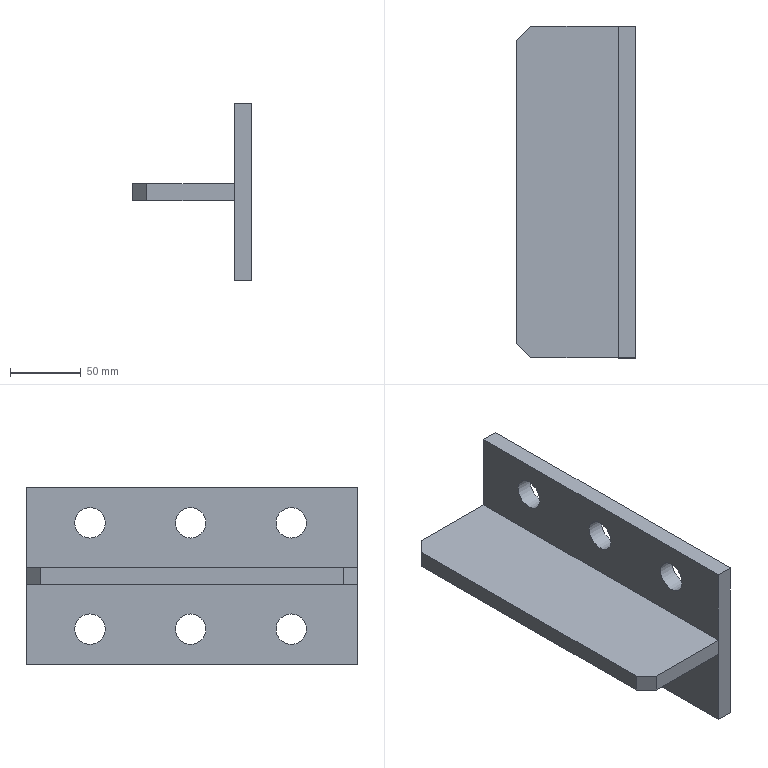Part | STEP file | PN_0028 web-top 12t steel corbel_Default<As Machined> | 2 solids | 20 faces | box 84 x 234 x 125 mm | volume 525836 mm3 | plane 14 | cylinder 6 | commonest cylinder face diameters 21.5 x6
STEP:
#1=CARTESIAN_POINT('',(0.,0.,0.));
#2=DIRECTION('',(0.,0.,1.));
#3=DIRECTION('',(1.,0.,0.));
#4=AXIS2_PLACEMENT_3D('',#1,#2,#3);
#5=CARTESIAN_POINT('',(-26.,117.,0.));
#6=VERTEX_POINT('',#5);
#7=CARTESIAN_POINT('',(-26.,117.,12.));
#8=VERTEX_POINT('',#7);
#9=CARTESIAN_POINT('',(-26.,117.,12.));
#10=DIRECTION('',(0.,0.,1.));
#11=VECTOR('',#10,1.);
#12=LINE('',#9,#11);
#13=CARTESIAN_POINT('',(-26.,117.,12.));
#14=DIRECTION('',(0.7071,-0.7071,0.));
#15=DIRECTION('',(0.,0.,1.));
#16=AXIS2_PLACEMENT_3D('',#13,#14,#15);
#17=PLANE('',#16);
#18=CARTESIAN_POINT('',(0.,0.));
#19=DIRECTION('',(1.,0.));
#20=VECTOR('',#19,1.);
#21=LINE('',#18,#20);
#22=(GEOMETRIC_REPRESENTATION_CONTEXT(2)PARAMETRIC_REPRESENTATION_CONTEXT()REPRESENTATION_CONTEXT('',''));
#23=DEFINITIONAL_REPRESENTATION('',(#21),#22);
#24=PCURVE('',#17,#23);
#25=CARTESIAN_POINT('',(-36.,117.,12.));
#26=DIRECTION('',(0.,-1.,0.));
#27=DIRECTION('',(0.,0.,-1.));
#28=AXIS2_PLACEMENT_3D('',#25,#26,#27);
#29=PLANE('',#28);
#30=CARTESIAN_POINT('',(0.,10.));
#31=DIRECTION('',(-1.,0.));
#32=VECTOR('',#31,1.);
#33=LINE('',#30,#32);
#34=(GEOMETRIC_REPRESENTATION_CONTEXT(2)PARAMETRIC_REPRESENTATION_CONTEXT()REPRESENTATION_CONTEXT('',''));
#35=DEFINITIONAL_REPRESENTATION('',(#33),#34);
#36=PCURVE('',#29,#35);
#37=SURFACE_CURVE('',#12,(#24,#36),.PCURVE_S1.);
#38=EDGE_CURVE('',#6,#8,#37,.T.);
#39=ORIENTED_EDGE('',*,*,#38,.F.);
#40=CARTESIAN_POINT('',(-36.,107.,0.));
#41=VERTEX_POINT('',#40);
#42=CARTESIAN_POINT('',(-26.,117.,0.));
#43=DIRECTION('',(0.7071,0.7071,0.));
#44=VECTOR('',#43,1.);
#45=LINE('',#42,#44);
#46=CARTESIAN_POINT('',(-12.,0.));
#47=DIRECTION('',(0.,-1.));
#48=VECTOR('',#47,1.);
#49=LINE('',#46,#48);
#50=(GEOMETRIC_REPRESENTATION_CONTEXT(2)PARAMETRIC_REPRESENTATION_CONTEXT()REPRESENTATION_CONTEXT('',''));
#51=DEFINITIONAL_REPRESENTATION('',(#49),#50);
#52=PCURVE('',#17,#51);
#53=CARTESIAN_POINT('',(0.,0.,0.));
#54=DIRECTION('',(0.,0.,1.));
#55=DIRECTION('',(1.,0.,0.));
#56=AXIS2_PLACEMENT_3D('',#53,#54,#55);
#57=PLANE('',#56);
#58=CARTESIAN_POINT('',(-26.,117.));
#59=DIRECTION('',(0.7071,0.7071));
#60=VECTOR('',#59,1.);
#61=LINE('',#58,#60);
#62=(GEOMETRIC_REPRESENTATION_CONTEXT(2)PARAMETRIC_REPRESENTATION_CONTEXT()REPRESENTATION_CONTEXT('',''));
#63=DEFINITIONAL_REPRESENTATION('',(#61),#62);
#64=PCURVE('',#57,#63);
#65=SURFACE_CURVE('',#45,(#52,#64),.PCURVE_S1.);
#66=EDGE_CURVE('',#41,#6,#65,.T.);
#67=ORIENTED_EDGE('',*,*,#66,.F.);
#68=CARTESIAN_POINT('',(-36.,107.,12.));
#69=VERTEX_POINT('',#68);
#70=CARTESIAN_POINT('',(-36.,107.,12.));
#71=DIRECTION('',(0.,0.,-1.));
#72=VECTOR('',#71,1.);
#73=LINE('',#70,#72);
#74=CARTESIAN_POINT('',(0.,14.142));
#75=DIRECTION('',(-1.,0.));
#76=VECTOR('',#75,1.);
#77=LINE('',#74,#76);
#78=(GEOMETRIC_REPRESENTATION_CONTEXT(2)PARAMETRIC_REPRESENTATION_CONTEXT()REPRESENTATION_CONTEXT('',''));
#79=DEFINITIONAL_REPRESENTATION('',(#77),#78);
#80=PCURVE('',#17,#79);
#81=CARTESIAN_POINT('',(-36.,117.,12.));
#82=DIRECTION('',(1.,0.,0.));
#83=DIRECTION('',(0.,0.,-1.));
#84=AXIS2_PLACEMENT_3D('',#81,#82,#83);
#85=PLANE('',#84);
#86=CARTESIAN_POINT('',(0.,-10.));
#87=DIRECTION('',(1.,0.));
#88=VECTOR('',#87,1.);
#89=LINE('',#86,#88);
#90=(GEOMETRIC_REPRESENTATION_CONTEXT(2)PARAMETRIC_REPRESENTATION_CONTEXT()REPRESENTATION_CONTEXT('',''));
#91=DEFINITIONAL_REPRESENTATION('',(#89),#90);
#92=PCURVE('',#85,#91);
#93=SURFACE_CURVE('',#73,(#80,#92),.PCURVE_S1.);
#94=EDGE_CURVE('',#69,#41,#93,.T.);
#95=ORIENTED_EDGE('',*,*,#94,.F.);
#96=CARTESIAN_POINT('',(-71.5,71.5,12.));
#97=DIRECTION('',(-0.7071,-0.7071,0.));
#98=VECTOR('',#97,1.);
#99=LINE('',#96,#98);
#100=CARTESIAN_POINT('',(0.,64.347));
#101=DIRECTION('',(0.,1.));
#102=VECTOR('',#101,1.);
#103=LINE('',#100,#102);
#104=(GEOMETRIC_REPRESENTATION_CONTEXT(2)PARAMETRIC_REPRESENTATION_CONTEXT()REPRESENTATION_CONTEXT('',''));
#105=DEFINITIONAL_REPRESENTATION('',(#103),#104);
#106=PCURVE('',#17,#105);
#107=CARTESIAN_POINT('',(0.,0.,12.));
#108=DIRECTION('',(0.,0.,1.));
#109=DIRECTION('',(1.,0.,0.));
#110=AXIS2_PLACEMENT_3D('',#107,#108,#109);
#111=PLANE('',#110);
#112=CARTESIAN_POINT('',(-71.5,71.5));
#113=DIRECTION('',(-0.7071,-0.7071));
#114=VECTOR('',#113,1.);
#115=LINE('',#112,#114);
#116=(GEOMETRIC_REPRESENTATION_CONTEXT(2)PARAMETRIC_REPRESENTATION_CONTEXT()REPRESENTATION_CONTEXT('',''));
#117=DEFINITIONAL_REPRESENTATION('',(#115),#116);
#118=PCURVE('',#111,#117);
#119=SURFACE_CURVE('',#99,(#106,#118),.PCURVE_S1.);
#120=EDGE_CURVE('',#8,#69,#119,.T.);
#121=ORIENTED_EDGE('',*,*,#120,.F.);
#122=EDGE_LOOP('',(#39,#67,#95,#121));
#123=FACE_BOUND('',#122,.T.);
#124=ADVANCED_FACE('',(#123),#17,.F.);
#125=CARTESIAN_POINT('',(-36.,-107.,0.));
#126=VERTEX_POINT('',#125);
#127=CARTESIAN_POINT('',(-36.,-107.,12.));
#128=VERTEX_POINT('',#127);
#129=CARTESIAN_POINT('',(-36.,-107.,12.));
#130=DIRECTION('',(0.,0.,1.));
#131=VECTOR('',#130,1.);
#132=LINE('',#129,#131);
#133=CARTESIAN_POINT('',(-36.,-107.,12.));
#134=DIRECTION('',(0.7071,0.7071,0.));
#135=DIRECTION('',(0.,0.,1.));
#136=AXIS2_PLACEMENT_3D('',#133,#134,#135);
#137=PLANE('',#136);
#138=CARTESIAN_POINT('',(0.,0.));
#139=DIRECTION('',(1.,0.));
#140=VECTOR('',#139,1.);
#141=LINE('',#138,#140);
#142=(GEOMETRIC_REPRESENTATION_CONTEXT(2)PARAMETRIC_REPRESENTATION_CONTEXT()REPRESENTATION_CONTEXT('',''));
#143=DEFINITIONAL_REPRESENTATION('',(#141),#142);
#144=PCURVE('',#137,#143);
#145=CARTESIAN_POINT('',(0.,-224.));
#146=DIRECTION('',(-1.,0.));
#147=VECTOR('',#146,1.);
#148=LINE('',#145,#147);
#149=(GEOMETRIC_REPRESENTATION_CONTEXT(2)PARAMETRIC_REPRESENTATION_CONTEXT()REPRESENTATION_CONTEXT('',''));
#150=DEFINITIONAL_REPRESENTATION('',(#148),#149);
#151=PCURVE('',#85,#150);
#152=SURFACE_CURVE('',#132,(#144,#151),.PCURVE_S1.);
#153=EDGE_CURVE('',#126,#128,#152,.T.);
#154=ORIENTED_EDGE('',*,*,#153,.F.);
#155=CARTESIAN_POINT('',(-26.,-117.,0.));
#156=VERTEX_POINT('',#155);
#157=CARTESIAN_POINT('',(-36.,-107.,0.));
#158=DIRECTION('',(-0.7071,0.7071,0.));
#159=VECTOR('',#158,1.);
#160=LINE('',#157,#159);
#161=CARTESIAN_POINT('',(-12.,0.));
#162=DIRECTION('',(0.,-1.));
#163=VECTOR('',#162,1.);
#164=LINE('',#161,#163);
#165=(GEOMETRIC_REPRESENTATION_CONTEXT(2)PARAMETRIC_REPRESENTATION_CONTEXT()REPRESENTATION_CONTEXT('',''));
#166=DEFINITIONAL_REPRESENTATION('',(#164),#165);
#167=PCURVE('',#137,#166);
#168=CARTESIAN_POINT('',(-36.,-107.));
#169=DIRECTION('',(-0.7071,0.7071));
#170=VECTOR('',#169,1.);
#171=LINE('',#168,#170);
#172=(GEOMETRIC_REPRESENTATION_CONTEXT(2)PARAMETRIC_REPRESENTATION_CONTEXT()REPRESENTATION_CONTEXT('',''));
#173=DEFINITIONAL_REPRESENTATION('',(#171),#172);
#174=PCURVE('',#57,#173);
#175=SURFACE_CURVE('',#160,(#167,#174),.PCURVE_S1.);
#176=EDGE_CURVE('',#156,#126,#175,.T.);
#177=ORIENTED_EDGE('',*,*,#176,.F.);
#178=CARTESIAN_POINT('',(-26.,-117.,12.));
#179=VERTEX_POINT('',#178);
#180=CARTESIAN_POINT('',(-26.,-117.,12.));
#181=DIRECTION('',(0.,0.,-1.));
#182=VECTOR('',#181,1.);
#183=LINE('',#180,#182);
#184=CARTESIAN_POINT('',(0.,14.142));
#185=DIRECTION('',(-1.,0.));
#186=VECTOR('',#185,1.);
#187=LINE('',#184,#186);
#188=(GEOMETRIC_REPRESENTATION_CONTEXT(2)PARAMETRIC_REPRESENTATION_CONTEXT()REPRESENTATION_CONTEXT('',''));
#189=DEFINITIONAL_REPRESENTATION('',(#187),#188);
#190=PCURVE('',#137,#189);
#191=CARTESIAN_POINT('',(-36.,-117.,12.));
#192=DIRECTION('',(0.,1.,0.));
#193=DIRECTION('',(0.,0.,1.));
#194=AXIS2_PLACEMENT_3D('',#191,#192,#193);
#195=PLANE('',#194);
#196=CARTESIAN_POINT('',(0.,10.));
#197=DIRECTION('',(-1.,0.));
#198=VECTOR('',#197,1.);
#199=LINE('',#196,#198);
#200=(GEOMETRIC_REPRESENTATION_CONTEXT(2)PARAMETRIC_REPRESENTATION_CONTEXT()REPRESENTATION_CONTEXT('',''));
#201=DEFINITIONAL_REPRESENTATION('',(#199),#200);
#202=PCURVE('',#195,#201);
#203=SURFACE_CURVE('',#183,(#190,#202),.PCURVE_S1.);
#204=EDGE_CURVE('',#179,#156,#203,.T.);
#205=ORIENTED_EDGE('',*,*,#204,.F.);
#206=CARTESIAN_POINT('',(-71.5,-71.5,12.));
#207=DIRECTION('',(0.7071,-0.7071,0.));
#208=VECTOR('',#207,1.);
#209=LINE('',#206,#208);
#210=CARTESIAN_POINT('',(0.,-50.205));
#211=DIRECTION('',(0.,1.));
#212=VECTOR('',#211,1.);
#213=LINE('',#210,#212);
#214=(GEOMETRIC_REPRESENTATION_CONTEXT(2)PARAMETRIC_REPRESENTATION_CONTEXT()REPRESENTATION_CONTEXT('',''));
#215=DEFINITIONAL_REPRESENTATION('',(#213),#214);
#216=PCURVE('',#137,#215);
#217=CARTESIAN_POINT('',(-71.5,-71.5));
#218=DIRECTION('',(0.7071,-0.7071));
#219=VECTOR('',#218,1.);
#220=LINE('',#217,#219);
#221=(GEOMETRIC_REPRESENTATION_CONTEXT(2)PARAMETRIC_REPRESENTATION_CONTEXT()REPRESENTATION_CONTEXT('',''));
#222=DEFINITIONAL_REPRESENTATION('',(#220),#221);
#223=PCURVE('',#111,#222);
#224=SURFACE_CURVE('',#209,(#216,#223),.PCURVE_S1.);
#225=EDGE_CURVE('',#128,#179,#224,.T.);
#226=ORIENTED_EDGE('',*,*,#225,.F.);
#227=EDGE_LOOP('',(#154,#177,#205,#226));
#228=FACE_BOUND('',#227,.T.);
#229=ADVANCED_FACE('',(#228),#137,.F.);
#230=CARTESIAN_POINT('',(36.,-117.,0.));
#231=VERTEX_POINT('',#230);
#232=CARTESIAN_POINT('',(36.,117.,0.));
#233=VERTEX_POINT('',#232);
#234=CARTESIAN_POINT('',(36.,117.,0.));
#235=DIRECTION('',(0.,1.,0.));
#236=VECTOR('',#235,1.);
#237=LINE('',#234,#236);
#238=CARTESIAN_POINT('',(36.,117.,12.));
#239=DIRECTION('',(-1.,0.,0.));
#240=DIRECTION('',(0.,0.,1.));
#241=AXIS2_PLACEMENT_3D('',#238,#239,#240);
#242=PLANE('',#241);
#243=CARTESIAN_POINT('',(-12.,0.));
#244=DIRECTION('',(0.,1.));
#245=VECTOR('',#244,1.);
#246=LINE('',#243,#245);
#247=(GEOMETRIC_REPRESENTATION_CONTEXT(2)PARAMETRIC_REPRESENTATION_CONTEXT()REPRESENTATION_CONTEXT('',''));
#248=DEFINITIONAL_REPRESENTATION('',(#246),#247);
#249=PCURVE('',#242,#248);
#250=CARTESIAN_POINT('',(36.,117.));
#251=DIRECTION('',(0.,1.));
#252=VECTOR('',#251,1.);
#253=LINE('',#250,#252);
#254=(GEOMETRIC_REPRESENTATION_CONTEXT(2)PARAMETRIC_REPRESENTATION_CONTEXT()REPRESENTATION_CONTEXT('',''));
#255=DEFINITIONAL_REPRESENTATION('',(#253),#254);
#256=PCURVE('',#57,#255);
#257=SURFACE_CURVE('',#237,(#249,#256),.PCURVE_S1.);
#258=EDGE_CURVE('',#231,#233,#257,.T.);
#259=ORIENTED_EDGE('',*,*,#258,.T.);
#260=CARTESIAN_POINT('',(36.,117.,12.));
#261=VERTEX_POINT('',#260);
#262=CARTESIAN_POINT('',(36.,117.,12.));
#263=DIRECTION('',(0.,0.,-1.));
#264=VECTOR('',#263,1.);
#265=LINE('',#262,#264);
#266=CARTESIAN_POINT('',(0.,0.));
#267=DIRECTION('',(-1.,0.));
#268=VECTOR('',#267,1.);
#269=LINE('',#266,#268);
#270=(GEOMETRIC_REPRESENTATION_CONTEXT(2)PARAMETRIC_REPRESENTATION_CONTEXT()REPRESENTATION_CONTEXT('',''));
#271=DEFINITIONAL_REPRESENTATION('',(#269),#270);
#272=PCURVE('',#242,#271);
#273=CARTESIAN_POINT('',(0.,72.));
#274=DIRECTION('',(1.,0.));
#275=VECTOR('',#274,1.);
#276=LINE('',#273,#275);
#277=(GEOMETRIC_REPRESENTATION_CONTEXT(2)PARAMETRIC_REPRESENTATION_CONTEXT()REPRESENTATION_CONTEXT('',''));
#278=DEFINITIONAL_REPRESENTATION('',(#276),#277);
#279=PCURVE('',#29,#278);
#280=SURFACE_CURVE('',#265,(#272,#279),.PCURVE_S1.);
#281=EDGE_CURVE('',#261,#233,#280,.T.);
#282=ORIENTED_EDGE('',*,*,#281,.F.);
#283=CARTESIAN_POINT('',(36.,-117.,12.));
#284=VERTEX_POINT('',#283);
#285=CARTESIAN_POINT('',(36.,117.,12.));
#286=DIRECTION('',(0.,1.,0.));
#287=VECTOR('',#286,1.);
#288=LINE('',#285,#287);
#289=CARTESIAN_POINT('',(0.,0.));
#290=DIRECTION('',(0.,1.));
#291=VECTOR('',#290,1.);
#292=LINE('',#289,#291);
#293=(GEOMETRIC_REPRESENTATION_CONTEXT(2)PARAMETRIC_REPRESENTATION_CONTEXT()REPRESENTATION_CONTEXT('',''));
#294=DEFINITIONAL_REPRESENTATION('',(#292),#293);
#295=PCURVE('',#242,#294);
#296=CARTESIAN_POINT('',(36.,117.));
#297=DIRECTION('',(0.,1.));
#298=VECTOR('',#297,1.);
#299=LINE('',#296,#298);
#300=(GEOMETRIC_REPRESENTATION_CONTEXT(2)PARAMETRIC_REPRESENTATION_CONTEXT()REPRESENTATION_CONTEXT('',''));
#301=DEFINITIONAL_REPRESENTATION('',(#299),#300);
#302=PCURVE('',#111,#301);
#303=SURFACE_CURVE('',#288,(#295,#302),.PCURVE_S1.);
#304=EDGE_CURVE('',#284,#261,#303,.T.);
#305=ORIENTED_EDGE('',*,*,#304,.F.);
#306=CARTESIAN_POINT('',(36.,-117.,12.));
#307=DIRECTION('',(0.,0.,-1.));
#308=VECTOR('',#307,1.);
#309=LINE('',#306,#308);
#310=CARTESIAN_POINT('',(0.,-234.));
#311=DIRECTION('',(-1.,0.));
#312=VECTOR('',#311,1.);
#313=LINE('',#310,#312);
#314=(GEOMETRIC_REPRESENTATION_CONTEXT(2)PARAMETRIC_REPRESENTATION_CONTEXT()REPRESENTATION_CONTEXT('',''));
#315=DEFINITIONAL_REPRESENTATION('',(#313),#314);
#316=PCURVE('',#242,#315);
#317=CARTESIAN_POINT('',(0.,72.));
#318=DIRECTION('',(-1.,0.));
#319=VECTOR('',#318,1.);
#320=LINE('',#317,#319);
#321=(GEOMETRIC_REPRESENTATION_CONTEXT(2)PARAMETRIC_REPRESENTATION_CONTEXT()REPRESENTATION_CONTEXT('',''));
#322=DEFINITIONAL_REPRESENTATION('',(#320),#321);
#323=PCURVE('',#195,#322);
#324=SURFACE_CURVE('',#309,(#316,#323),.PCURVE_S1.);
#325=EDGE_CURVE('',#284,#231,#324,.T.);
#326=ORIENTED_EDGE('',*,*,#325,.T.);
#327=EDGE_LOOP('',(#259,#282,#305,#326));
#328=FACE_BOUND('',#327,.T.);
#329=ADVANCED_FACE('',(#328),#242,.F.);
#330=CARTESIAN_POINT('',(-36.,117.,0.));
#331=DIRECTION('',(-1.,0.,0.));
#332=VECTOR('',#331,1.);
#333=LINE('',#330,#332);
#334=CARTESIAN_POINT('',(12.,0.));
#335=DIRECTION('',(0.,-1.));
#336=VECTOR('',#335,1.);
#337=LINE('',#334,#336);
#338=(GEOMETRIC_REPRESENTATION_CONTEXT(2)PARAMETRIC_REPRESENTATION_CONTEXT()REPRESENTATION_CONTEXT('',''));
#339=DEFINITIONAL_REPRESENTATION('',(#337),#338);
#340=PCURVE('',#29,#339);
#341=CARTESIAN_POINT('',(-36.,117.));
#342=DIRECTION('',(-1.,0.));
#343=VECTOR('',#342,1.);
#344=LINE('',#341,#343);
#345=(GEOMETRIC_REPRESENTATION_CONTEXT(2)PARAMETRIC_REPRESENTATION_CONTEXT()REPRESENTATION_CONTEXT('',''));
#346=DEFINITIONAL_REPRESENTATION('',(#344),#345);
#347=PCURVE('',#57,#346);
#348=SURFACE_CURVE('',#333,(#340,#347),.PCURVE_S1.);
#349=EDGE_CURVE('',#233,#6,#348,.T.);
#350=ORIENTED_EDGE('',*,*,#349,.T.);
#351=ORIENTED_EDGE('',*,*,#38,.T.);
#352=CARTESIAN_POINT('',(-36.,117.,12.));
#353=DIRECTION('',(-1.,0.,0.));
#354=VECTOR('',#353,1.);
#355=LINE('',#352,#354);
#356=CARTESIAN_POINT('',(0.,0.));
#357=DIRECTION('',(0.,-1.));
#358=VECTOR('',#357,1.);
#359=LINE('',#356,#358);
#360=(GEOMETRIC_REPRESENTATION_CONTEXT(2)PARAMETRIC_REPRESENTATION_CONTEXT()REPRESENTATION_CONTEXT('',''));
#361=DEFINITIONAL_REPRESENTATION('',(#359),#360);
#362=PCURVE('',#29,#361);
#363=CARTESIAN_POINT('',(-36.,117.));
#364=DIRECTION('',(-1.,0.));
#365=VECTOR('',#364,1.);
#366=LINE('',#363,#365);
#367=(GEOMETRIC_REPRESENTATION_CONTEXT(2)PARAMETRIC_REPRESENTATION_CONTEXT()REPRESENTATION_CONTEXT('',''));
#368=DEFINITIONAL_REPRESENTATION('',(#366),#367);
#369=PCURVE('',#111,#368);
#370=SURFACE_CURVE('',#355,(#362,#369),.PCURVE_S1.);
#371=EDGE_CURVE('',#261,#8,#370,.T.);
#372=ORIENTED_EDGE('',*,*,#371,.F.);
#373=ORIENTED_EDGE('',*,*,#281,.T.);
#374=EDGE_LOOP('',(#350,#351,#372,#373));
#375=FACE_BOUND('',#374,.T.);
#376=ADVANCED_FACE('',(#375),#29,.F.);
#377=CARTESIAN_POINT('',(-36.,117.,12.));
#378=DIRECTION('',(0.,-1.,0.));
#379=VECTOR('',#378,1.);
#380=LINE('',#377,#379);
#381=CARTESIAN_POINT('',(0.,0.));
#382=DIRECTION('',(0.,-1.));
#383=VECTOR('',#382,1.);
#384=LINE('',#381,#383);
#385=(GEOMETRIC_REPRESENTATION_CONTEXT(2)PARAMETRIC_REPRESENTATION_CONTEXT()REPRESENTATION_CONTEXT('',''));
#386=DEFINITIONAL_REPRESENTATION('',(#384),#385);
#387=PCURVE('',#85,#386);
#388=CARTESIAN_POINT('',(-36.,117.));
#389=DIRECTION('',(0.,-1.));
#390=VECTOR('',#389,1.);
#391=LINE('',#388,#390);
#392=(GEOMETRIC_REPRESENTATION_CONTEXT(2)PARAMETRIC_REPRESENTATION_CONTEXT()REPRESENTATION_CONTEXT('',''));
#393=DEFINITIONAL_REPRESENTATION('',(#391),#392);
#394=PCURVE('',#111,#393);
#395=SURFACE_CURVE('',#380,(#387,#394),.PCURVE_S1.);
#396=EDGE_CURVE('',#69,#128,#395,.T.);
#397=ORIENTED_EDGE('',*,*,#396,.F.);
#398=ORIENTED_EDGE('',*,*,#94,.T.);
#399=CARTESIAN_POINT('',(-36.,117.,0.));
#400=DIRECTION('',(0.,-1.,0.));
#401=VECTOR('',#400,1.);
#402=LINE('',#399,#401);
#403=CARTESIAN_POINT('',(12.,0.));
#404=DIRECTION('',(0.,-1.));
#405=VECTOR('',#404,1.);
#406=LINE('',#403,#405);
#407=(GEOMETRIC_REPRESENTATION_CONTEXT(2)PARAMETRIC_REPRESENTATION_CONTEXT()REPRESENTATION_CONTEXT('',''));
#408=DEFINITIONAL_REPRESENTATION('',(#406),#407);
#409=PCURVE('',#85,#408);
#410=CARTESIAN_POINT('',(-36.,117.));
#411=DIRECTION('',(0.,-1.));
#412=VECTOR('',#411,1.);
#413=LINE('',#410,#412);
#414=(GEOMETRIC_REPRESENTATION_CONTEXT(2)PARAMETRIC_REPRESENTATION_CONTEXT()REPRESENTATION_CONTEXT('',''));
#415=DEFINITIONAL_REPRESENTATION('',(#413),#414);
#416=PCURVE('',#57,#415);
#417=SURFACE_CURVE('',#402,(#409,#416),.PCURVE_S1.);
#418=EDGE_CURVE('',#41,#126,#417,.T.);
#419=ORIENTED_EDGE('',*,*,#418,.T.);
#420=ORIENTED_EDGE('',*,*,#153,.T.);
#421=EDGE_LOOP('',(#397,#398,#419,#420));
#422=FACE_BOUND('',#421,.T.);
#423=ADVANCED_FACE('',(#422),#85,.F.);
#424=CARTESIAN_POINT('',(-36.,-117.,12.));
#425=DIRECTION('',(1.,0.,0.));
#426=VECTOR('',#425,1.);
#427=LINE('',#424,#426);
#428=CARTESIAN_POINT('',(0.,0.));
#429=DIRECTION('',(0.,1.));
#430=VECTOR('',#429,1.);
#431=LINE('',#428,#430);
#432=(GEOMETRIC_REPRESENTATION_CONTEXT(2)PARAMETRIC_REPRESENTATION_CONTEXT()REPRESENTATION_CONTEXT('',''));
#433=DEFINITIONAL_REPRESENTATION('',(#431),#432);
#434=PCURVE('',#195,#433);
#435=CARTESIAN_POINT('',(-36.,-117.));
#436=DIRECTION('',(1.,0.));
#437=VECTOR('',#436,1.);
#438=LINE('',#435,#437);
#439=(GEOMETRIC_REPRESENTATION_CONTEXT(2)PARAMETRIC_REPRESENTATION_CONTEXT()REPRESENTATION_CONTEXT('',''));
#440=DEFINITIONAL_REPRESENTATION('',(#438),#439);
#441=PCURVE('',#111,#440);
#442=SURFACE_CURVE('',#427,(#434,#441),.PCURVE_S1.);
#443=EDGE_CURVE('',#179,#284,#442,.T.);
#444=ORIENTED_EDGE('',*,*,#443,.F.);
#445=ORIENTED_EDGE('',*,*,#204,.T.);
#446=CARTESIAN_POINT('',(-36.,-117.,0.));
#447=DIRECTION('',(1.,0.,0.));
#448=VECTOR('',#447,1.);
#449=LINE('',#446,#448);
#450=CARTESIAN_POINT('',(-12.,0.));
#451=DIRECTION('',(0.,1.));
#452=VECTOR('',#451,1.);
#453=LINE('',#450,#452);
#454=(GEOMETRIC_REPRESENTATION_CONTEXT(2)PARAMETRIC_REPRESENTATION_CONTEXT()REPRESENTATION_CONTEXT('',''));
#455=DEFINITIONAL_REPRESENTATION('',(#453),#454);
#456=PCURVE('',#195,#455);
#457=CARTESIAN_POINT('',(-36.,-117.));
#458=DIRECTION('',(1.,0.));
#459=VECTOR('',#458,1.);
#460=LINE('',#457,#459);
#461=(GEOMETRIC_REPRESENTATION_CONTEXT(2)PARAMETRIC_REPRESENTATION_CONTEXT()REPRESENTATION_CONTEXT('',''));
#462=DEFINITIONAL_REPRESENTATION('',(#460),#461);
#463=PCURVE('',#57,#462);
#464=SURFACE_CURVE('',#449,(#456,#463),.PCURVE_S1.);
#465=EDGE_CURVE('',#156,#231,#464,.T.);
#466=ORIENTED_EDGE('',*,*,#465,.T.);
#467=ORIENTED_EDGE('',*,*,#325,.F.);
#468=EDGE_LOOP('',(#444,#445,#466,#467));
#469=FACE_BOUND('',#468,.T.);
#470=ADVANCED_FACE('',(#469),#195,.F.);
#471=ORIENTED_EDGE('',*,*,#371,.T.);
#472=ORIENTED_EDGE('',*,*,#120,.T.);
#473=ORIENTED_EDGE('',*,*,#396,.T.);
#474=ORIENTED_EDGE('',*,*,#225,.T.);
#475=ORIENTED_EDGE('',*,*,#443,.T.);
#476=ORIENTED_EDGE('',*,*,#304,.T.);
#477=EDGE_LOOP('',(#471,#472,#473,#474,#475,#476));
#478=FACE_BOUND('',#477,.T.);
#479=ADVANCED_FACE('',(#478),#111,.T.);
#480=ORIENTED_EDGE('',*,*,#418,.F.);
#481=ORIENTED_EDGE('',*,*,#66,.T.);
#482=ORIENTED_EDGE('',*,*,#349,.F.);
#483=ORIENTED_EDGE('',*,*,#258,.F.);
#484=ORIENTED_EDGE('',*,*,#465,.F.);
#485=ORIENTED_EDGE('',*,*,#176,.T.);
#486=EDGE_LOOP('',(#480,#481,#482,#483,#484,#485));
#487=FACE_BOUND('',#486,.T.);
#488=ADVANCED_FACE('',(#487),#57,.F.);
#489=CLOSED_SHELL('',(#124,#229,#329,#376,#423,#470,#479,#488));
#490=MANIFOLD_SOLID_BREP('',#489);
#491=CARTESIAN_POINT('',(36.,-117.,-56.496));
#492=VERTEX_POINT('',#491);
#493=CARTESIAN_POINT('',(36.,117.,-56.496));
#494=VERTEX_POINT('',#493);
#495=CARTESIAN_POINT('',(36.,117.,-56.496));
#496=DIRECTION('',(0.,1.,0.));
#497=VECTOR('',#496,1.);
#498=LINE('',#495,#497);
#499=CARTESIAN_POINT('',(48.,117.,-56.496));
#500=DIRECTION('',(0.,0.,1.));
#501=DIRECTION('',(1.,0.,0.));
#502=AXIS2_PLACEMENT_3D('',#499,#500,#501);
#503=PLANE('',#502);
#504=CARTESIAN_POINT('',(-12.,0.));
#505=DIRECTION('',(0.,1.));
#506=VECTOR('',#505,1.);
#507=LINE('',#504,#506);
#508=(GEOMETRIC_REPRESENTATION_CONTEXT(2)PARAMETRIC_REPRESENTATION_CONTEXT()REPRESENTATION_CONTEXT('',''));
#509=DEFINITIONAL_REPRESENTATION('',(#507),#508);
#510=PCURVE('',#503,#509);
#511=CARTESIAN_POINT('',(36.,-17.06,106.06));
#512=DIRECTION('',(1.,0.,0.));
#513=DIRECTION('',(0.,0.,-1.));
#514=AXIS2_PLACEMENT_3D('',#511,#512,#513);
#515=PLANE('',#514);
#516=CARTESIAN_POINT('',(162.556,134.06));
#517=DIRECTION('',(0.,1.));
#518=VECTOR('',#517,1.);
#519=LINE('',#516,#518);
#520=(GEOMETRIC_REPRESENTATION_CONTEXT(2)PARAMETRIC_REPRESENTATION_CONTEXT()REPRESENTATION_CONTEXT('',''));
#521=DEFINITIONAL_REPRESENTATION('',(#519),#520);
#522=PCURVE('',#515,#521);
#523=SURFACE_CURVE('',#498,(#510,#522),.PCURVE_S1.);
#524=EDGE_CURVE('',#492,#494,#523,.T.);
#525=ORIENTED_EDGE('',*,*,#524,.T.);
#526=CARTESIAN_POINT('',(48.,117.,-56.496));
#527=VERTEX_POINT('',#526);
#528=CARTESIAN_POINT('',(48.,117.,-56.496));
#529=DIRECTION('',(-1.,0.,0.));
#530=VECTOR('',#529,1.);
#531=LINE('',#528,#530);
#532=CARTESIAN_POINT('',(0.,0.));
#533=DIRECTION('',(-1.,0.));
#534=VECTOR('',#533,1.);
#535=LINE('',#532,#534);
#536=(GEOMETRIC_REPRESENTATION_CONTEXT(2)PARAMETRIC_REPRESENTATION_CONTEXT()REPRESENTATION_CONTEXT('',''));
#537=DEFINITIONAL_REPRESENTATION('',(#535),#536);
#538=PCURVE('',#503,#537);
#539=CARTESIAN_POINT('',(48.,117.,68.504));
#540=DIRECTION('',(0.,-1.,0.));
#541=DIRECTION('',(0.,0.,-1.));
#542=AXIS2_PLACEMENT_3D('',#539,#540,#541);
#543=PLANE('',#542);
#544=CARTESIAN_POINT('',(125.,0.));
#545=DIRECTION('',(0.,-1.));
#546=VECTOR('',#545,1.);
#547=LINE('',#544,#546);
#548=(GEOMETRIC_REPRESENTATION_CONTEXT(2)PARAMETRIC_REPRESENTATION_CONTEXT()REPRESENTATION_CONTEXT('',''));
#549=DEFINITIONAL_REPRESENTATION('',(#547),#548);
#550=PCURVE('',#543,#549);
#551=SURFACE_CURVE('',#531,(#538,#550),.PCURVE_S1.);
#552=EDGE_CURVE('',#527,#494,#551,.T.);
#553=ORIENTED_EDGE('',*,*,#552,.F.);
#554=CARTESIAN_POINT('',(48.,-117.,-56.496));
#555=VERTEX_POINT('',#554);
#556=CARTESIAN_POINT('',(48.,117.,-56.496));
#557=DIRECTION('',(0.,1.,0.));
#558=VECTOR('',#557,1.);
#559=LINE('',#556,#558);
#560=CARTESIAN_POINT('',(0.,0.));
#561=DIRECTION('',(0.,1.));
#562=VECTOR('',#561,1.);
#563=LINE('',#560,#562);
#564=(GEOMETRIC_REPRESENTATION_CONTEXT(2)PARAMETRIC_REPRESENTATION_CONTEXT()REPRESENTATION_CONTEXT('',''));
#565=DEFINITIONAL_REPRESENTATION('',(#563),#564);
#566=PCURVE('',#503,#565);
#567=CARTESIAN_POINT('',(48.,-17.06,106.06));
#568=DIRECTION('',(1.,0.,0.));
#569=DIRECTION('',(0.,0.,-1.));
#570=AXIS2_PLACEMENT_3D('',#567,#568,#569);
#571=PLANE('',#570);
#572=CARTESIAN_POINT('',(162.556,134.06));
#573=DIRECTION('',(0.,1.));
#574=VECTOR('',#573,1.);
#575=LINE('',#572,#574);
#576=(GEOMETRIC_REPRESENTATION_CONTEXT(2)PARAMETRIC_REPRESENTATION_CONTEXT()REPRESENTATION_CONTEXT('',''));
#577=DEFINITIONAL_REPRESENTATION('',(#575),#576);
#578=PCURVE('',#571,#577);
#579=SURFACE_CURVE('',#559,(#566,#578),.PCURVE_S1.);
#580=EDGE_CURVE('',#555,#527,#579,.T.);
#581=ORIENTED_EDGE('',*,*,#580,.F.);
#582=CARTESIAN_POINT('',(48.,-117.,-56.496));
#583=DIRECTION('',(-1.,0.,0.));
#584=VECTOR('',#583,1.);
#585=LINE('',#582,#584);
#586=CARTESIAN_POINT('',(0.,-234.));
#587=DIRECTION('',(-1.,0.));
#588=VECTOR('',#587,1.);
#589=LINE('',#586,#588);
#590=(GEOMETRIC_REPRESENTATION_CONTEXT(2)PARAMETRIC_REPRESENTATION_CONTEXT()REPRESENTATION_CONTEXT('',''));
#591=DEFINITIONAL_REPRESENTATION('',(#589),#590);
#592=PCURVE('',#503,#591);
#593=CARTESIAN_POINT('',(48.,-117.,68.504));
#594=DIRECTION('',(0.,1.,0.));
#595=DIRECTION('',(0.,0.,1.));
#596=AXIS2_PLACEMENT_3D('',#593,#594,#595);
#597=PLANE('',#596);
#598=CARTESIAN_POINT('',(-125.,0.));
#599=DIRECTION('',(0.,-1.));
#600=VECTOR('',#599,1.);
#601=LINE('',#598,#600);
#602=(GEOMETRIC_REPRESENTATION_CONTEXT(2)PARAMETRIC_REPRESENTATION_CONTEXT()REPRESENTATION_CONTEXT('',''));
#603=DEFINITIONAL_REPRESENTATION('',(#601),#602);
#604=PCURVE('',#597,#603);
#605=SURFACE_CURVE('',#585,(#592,#604),.PCURVE_S1.);
#606=EDGE_CURVE('',#555,#492,#605,.T.);
#607=ORIENTED_EDGE('',*,*,#606,.T.);
#608=EDGE_LOOP('',(#525,#553,#581,#607));
#609=FACE_BOUND('',#608,.T.);
#610=ADVANCED_FACE('',(#609),#503,.F.);
#611=CARTESIAN_POINT('',(36.,117.,68.504));
#612=VERTEX_POINT('',#611);
#613=CARTESIAN_POINT('',(36.,117.,68.504));
#614=DIRECTION('',(0.,0.,1.));
#615=VECTOR('',#614,1.);
#616=LINE('',#613,#615);
#617=CARTESIAN_POINT('',(0.,-12.));
#618=DIRECTION('',(-1.,0.));
#619=VECTOR('',#618,1.);
#620=LINE('',#617,#619);
#621=(GEOMETRIC_REPRESENTATION_CONTEXT(2)PARAMETRIC_REPRESENTATION_CONTEXT()REPRESENTATION_CONTEXT('',''));
#622=DEFINITIONAL_REPRESENTATION('',(#620),#621);
#623=PCURVE('',#543,#622);
#624=CARTESIAN_POINT('',(37.556,134.06));
#625=DIRECTION('',(-1.,0.));
#626=VECTOR('',#625,1.);
#627=LINE('',#624,#626);
#628=(GEOMETRIC_REPRESENTATION_CONTEXT(2)PARAMETRIC_REPRESENTATION_CONTEXT()REPRESENTATION_CONTEXT('',''));
#629=DEFINITIONAL_REPRESENTATION('',(#627),#628);
#630=PCURVE('',#515,#629);
#631=SURFACE_CURVE('',#616,(#623,#630),.PCURVE_S1.);
#632=EDGE_CURVE('',#494,#612,#631,.T.);
#633=ORIENTED_EDGE('',*,*,#632,.T.);
#634=CARTESIAN_POINT('',(48.,117.,68.504));
#635=VERTEX_POINT('',#634);
#636=CARTESIAN_POINT('',(48.,117.,68.504));
#637=DIRECTION('',(-1.,0.,0.));
#638=VECTOR('',#637,1.);
#639=LINE('',#636,#638);
#640=CARTESIAN_POINT('',(0.,0.));
#641=DIRECTION('',(0.,-1.));
#642=VECTOR('',#641,1.);
#643=LINE('',#640,#642);
#644=(GEOMETRIC_REPRESENTATION_CONTEXT(2)PARAMETRIC_REPRESENTATION_CONTEXT()REPRESENTATION_CONTEXT('',''));
#645=DEFINITIONAL_REPRESENTATION('',(#643),#644);
#646=PCURVE('',#543,#645);
#647=CARTESIAN_POINT('',(48.,117.,68.504));
#648=DIRECTION('',(0.,0.,-1.));
#649=DIRECTION('',(0.,1.,0.));
#650=AXIS2_PLACEMENT_3D('',#647,#648,#649);
#651=PLANE('',#650);
#652=CARTESIAN_POINT('',(0.,0.));
#653=DIRECTION('',(0.,-1.));
#654=VECTOR('',#653,1.);
#655=LINE('',#652,#654);
#656=(GEOMETRIC_REPRESENTATION_CONTEXT(2)PARAMETRIC_REPRESENTATION_CONTEXT()REPRESENTATION_CONTEXT('',''));
#657=DEFINITIONAL_REPRESENTATION('',(#655),#656);
#658=PCURVE('',#651,#657);
#659=SURFACE_CURVE('',#639,(#646,#658),.PCURVE_S1.);
#660=EDGE_CURVE('',#635,#612,#659,.T.);
#661=ORIENTED_EDGE('',*,*,#660,.F.);
#662=CARTESIAN_POINT('',(48.,117.,68.504));
#663=DIRECTION('',(0.,0.,1.));
#664=VECTOR('',#663,1.);
#665=LINE('',#662,#664);
#666=CARTESIAN_POINT('',(0.,0.));
#667=DIRECTION('',(-1.,0.));
#668=VECTOR('',#667,1.);
#669=LINE('',#666,#668);
#670=(GEOMETRIC_REPRESENTATION_CONTEXT(2)PARAMETRIC_REPRESENTATION_CONTEXT()REPRESENTATION_CONTEXT('',''));
#671=DEFINITIONAL_REPRESENTATION('',(#669),#670);
#672=PCURVE('',#543,#671);
#673=CARTESIAN_POINT('',(37.556,134.06));
#674=DIRECTION('',(-1.,0.));
#675=VECTOR('',#674,1.);
#676=LINE('',#673,#675);
#677=(GEOMETRIC_REPRESENTATION_CONTEXT(2)PARAMETRIC_REPRESENTATION_CONTEXT()REPRESENTATION_CONTEXT('',''));
#678=DEFINITIONAL_REPRESENTATION('',(#676),#677);
#679=PCURVE('',#571,#678);
#680=SURFACE_CURVE('',#665,(#672,#679),.PCURVE_S1.);
#681=EDGE_CURVE('',#527,#635,#680,.T.);
#682=ORIENTED_EDGE('',*,*,#681,.F.);
#683=ORIENTED_EDGE('',*,*,#552,.T.);
#684=EDGE_LOOP('',(#633,#661,#682,#683));
#685=FACE_BOUND('',#684,.T.);
#686=ADVANCED_FACE('',(#685),#543,.F.);
#687=CARTESIAN_POINT('',(36.,-117.,68.504));
#688=VERTEX_POINT('',#687);
#689=CARTESIAN_POINT('',(36.,117.,68.504));
#690=DIRECTION('',(0.,-1.,0.));
#691=VECTOR('',#690,1.);
#692=LINE('',#689,#691);
#693=CARTESIAN_POINT('',(0.,-12.));
#694=DIRECTION('',(-1.,0.));
#695=VECTOR('',#694,1.);
#696=LINE('',#693,#695);
#697=(GEOMETRIC_REPRESENTATION_CONTEXT(2)PARAMETRIC_REPRESENTATION_CONTEXT()REPRESENTATION_CONTEXT('',''));
#698=DEFINITIONAL_REPRESENTATION('',(#696),#697);
#699=PCURVE('',#651,#698);
#700=CARTESIAN_POINT('',(37.556,134.06));
#701=DIRECTION('',(0.,-1.));
#702=VECTOR('',#701,1.);
#703=LINE('',#700,#702);
#704=(GEOMETRIC_REPRESENTATION_CONTEXT(2)PARAMETRIC_REPRESENTATION_CONTEXT()REPRESENTATION_CONTEXT('',''));
#705=DEFINITIONAL_REPRESENTATION('',(#703),#704);
#706=PCURVE('',#515,#705);
#707=SURFACE_CURVE('',#692,(#699,#706),.PCURVE_S1.);
#708=EDGE_CURVE('',#612,#688,#707,.T.);
#709=ORIENTED_EDGE('',*,*,#708,.T.);
#710=CARTESIAN_POINT('',(48.,-117.,68.504));
#711=VERTEX_POINT('',#710);
#712=CARTESIAN_POINT('',(48.,-117.,68.504));
#713=DIRECTION('',(-1.,0.,0.));
#714=VECTOR('',#713,1.);
#715=LINE('',#712,#714);
#716=CARTESIAN_POINT('',(-234.,0.));
#717=DIRECTION('',(0.,-1.));
#718=VECTOR('',#717,1.);
#719=LINE('',#716,#718);
#720=(GEOMETRIC_REPRESENTATION_CONTEXT(2)PARAMETRIC_REPRESENTATION_CONTEXT()REPRESENTATION_CONTEXT('',''));
#721=DEFINITIONAL_REPRESENTATION('',(#719),#720);
#722=PCURVE('',#651,#721);
#723=CARTESIAN_POINT('',(0.,0.));
#724=DIRECTION('',(0.,-1.));
#725=VECTOR('',#724,1.);
#726=LINE('',#723,#725);
#727=(GEOMETRIC_REPRESENTATION_CONTEXT(2)PARAMETRIC_REPRESENTATION_CONTEXT()REPRESENTATION_CONTEXT('',''));
#728=DEFINITIONAL_REPRESENTATION('',(#726),#727);
#729=PCURVE('',#597,#728);
#730=SURFACE_CURVE('',#715,(#722,#729),.PCURVE_S1.);
#731=EDGE_CURVE('',#711,#688,#730,.T.);
#732=ORIENTED_EDGE('',*,*,#731,.F.);
#733=CARTESIAN_POINT('',(48.,117.,68.504));
#734=DIRECTION('',(0.,-1.,0.));
#735=VECTOR('',#734,1.);
#736=LINE('',#733,#735);
#737=CARTESIAN_POINT('',(0.,0.));
#738=DIRECTION('',(-1.,0.));
#739=VECTOR('',#738,1.);
#740=LINE('',#737,#739);
#741=(GEOMETRIC_REPRESENTATION_CONTEXT(2)PARAMETRIC_REPRESENTATION_CONTEXT()REPRESENTATION_CONTEXT('',''));
#742=DEFINITIONAL_REPRESENTATION('',(#740),#741);
#743=PCURVE('',#651,#742);
#744=CARTESIAN_POINT('',(37.556,134.06));
#745=DIRECTION('',(0.,-1.));
#746=VECTOR('',#745,1.);
#747=LINE('',#744,#746);
#748=(GEOMETRIC_REPRESENTATION_CONTEXT(2)PARAMETRIC_REPRESENTATION_CONTEXT()REPRESENTATION_CONTEXT('',''));
#749=DEFINITIONAL_REPRESENTATION('',(#747),#748);
#750=PCURVE('',#571,#749);
#751=SURFACE_CURVE('',#736,(#743,#750),.PCURVE_S1.);
#752=EDGE_CURVE('',#635,#711,#751,.T.);
#753=ORIENTED_EDGE('',*,*,#752,.F.);
#754=ORIENTED_EDGE('',*,*,#660,.T.);
#755=EDGE_LOOP('',(#709,#732,#753,#754));
#756=FACE_BOUND('',#755,.T.);
#757=ADVANCED_FACE('',(#756),#651,.F.);
#758=CARTESIAN_POINT('',(36.,-117.,68.504));
#759=DIRECTION('',(0.,0.,-1.));
#760=VECTOR('',#759,1.);
#761=LINE('',#758,#760);
#762=CARTESIAN_POINT('',(0.,-12.));
#763=DIRECTION('',(-1.,0.));
#764=VECTOR('',#763,1.);
#765=LINE('',#762,#764);
#766=(GEOMETRIC_REPRESENTATION_CONTEXT(2)PARAMETRIC_REPRESENTATION_CONTEXT()REPRESENTATION_CONTEXT('',''));
#767=DEFINITIONAL_REPRESENTATION('',(#765),#766);
#768=PCURVE('',#597,#767);
#769=CARTESIAN_POINT('',(37.556,-99.94));
#770=DIRECTION('',(1.,0.));
#771=VECTOR('',#770,1.);
#772=LINE('',#769,#771);
#773=(GEOMETRIC_REPRESENTATION_CONTEXT(2)PARAMETRIC_REPRESENTATION_CONTEXT()REPRESENTATION_CONTEXT('',''));
#774=DEFINITIONAL_REPRESENTATION('',(#772),#773);
#775=PCURVE('',#515,#774);
#776=SURFACE_CURVE('',#761,(#768,#775),.PCURVE_S1.);
#777=EDGE_CURVE('',#688,#492,#776,.T.);
#778=ORIENTED_EDGE('',*,*,#777,.T.);
#779=ORIENTED_EDGE('',*,*,#606,.F.);
#780=CARTESIAN_POINT('',(48.,-117.,68.504));
#781=DIRECTION('',(0.,0.,-1.));
#782=VECTOR('',#781,1.);
#783=LINE('',#780,#782);
#784=CARTESIAN_POINT('',(0.,0.));
#785=DIRECTION('',(-1.,0.));
#786=VECTOR('',#785,1.);
#787=LINE('',#784,#786);
#788=(GEOMETRIC_REPRESENTATION_CONTEXT(2)PARAMETRIC_REPRESENTATION_CONTEXT()REPRESENTATION_CONTEXT('',''));
#789=DEFINITIONAL_REPRESENTATION('',(#787),#788);
#790=PCURVE('',#597,#789);
#791=CARTESIAN_POINT('',(37.556,-99.94));
#792=DIRECTION('',(1.,0.));
#793=VECTOR('',#792,1.);
#794=LINE('',#791,#793);
#795=(GEOMETRIC_REPRESENTATION_CONTEXT(2)PARAMETRIC_REPRESENTATION_CONTEXT()REPRESENTATION_CONTEXT('',''));
#796=DEFINITIONAL_REPRESENTATION('',(#794),#795);
#797=PCURVE('',#571,#796);
#798=SURFACE_CURVE('',#783,(#790,#797),.PCURVE_S1.);
#799=EDGE_CURVE('',#711,#555,#798,.T.);
#800=ORIENTED_EDGE('',*,*,#799,.F.);
#801=ORIENTED_EDGE('',*,*,#731,.T.);
#802=EDGE_LOOP('',(#778,#779,#800,#801));
#803=FACE_BOUND('',#802,.T.);
#804=ADVANCED_FACE('',(#803),#597,.F.);
#805=CARTESIAN_POINT('',(48.,72.,32.754));
#806=VERTEX_POINT('',#805);
#807=CARTESIAN_POINT('',(48.,72.,43.504));
#808=DIRECTION('',(1.,0.,0.));
#809=DIRECTION('',(0.,0.,-1.));
#810=AXIS2_PLACEMENT_3D('',#807,#808,#809);
#811=CIRCLE('',#810,10.75);
#812=CARTESIAN_POINT('',(62.556,89.06));
#813=DIRECTION('',(1.,0.));
#814=AXIS2_PLACEMENT_2D('',#812,#813);
#815=CIRCLE('',#814,10.75);
#816=(GEOMETRIC_REPRESENTATION_CONTEXT(2)PARAMETRIC_REPRESENTATION_CONTEXT()REPRESENTATION_CONTEXT('',''));
#817=DEFINITIONAL_REPRESENTATION('',(#815),#816);
#818=PCURVE('',#571,#817);
#819=CARTESIAN_POINT('',(48.,72.,43.504));
#820=DIRECTION('',(1.,0.,0.));
#821=DIRECTION('',(0.,0.,-1.));
#822=AXIS2_PLACEMENT_3D('',#819,#820,#821);
#823=CYLINDRICAL_SURFACE('',#822,10.75);
#824=CARTESIAN_POINT('',(0.,0.));
#825=DIRECTION('',(1.,0.));
#826=VECTOR('',#825,1.);
#827=LINE('',#824,#826);
#828=(GEOMETRIC_REPRESENTATION_CONTEXT(2)PARAMETRIC_REPRESENTATION_CONTEXT()REPRESENTATION_CONTEXT('',''));
#829=DEFINITIONAL_REPRESENTATION('',(#827),#828);
#830=PCURVE('',#823,#829);
#831=SURFACE_CURVE('',#811,(#818,#830),.PCURVE_S1.);
#832=EDGE_CURVE('',#806,#806,#831,.T.);
#833=ORIENTED_EDGE('',*,*,#832,.F.);
#834=EDGE_LOOP('',(#833));
#835=FACE_BOUND('',#834,.T.);
#836=CARTESIAN_POINT('',(48.,1.,32.754));
#837=VERTEX_POINT('',#836);
#838=CARTESIAN_POINT('',(48.,1.,43.504));
#839=DIRECTION('',(1.,0.,0.));
#840=DIRECTION('',(0.,0.,-1.));
#841=AXIS2_PLACEMENT_3D('',#838,#839,#840);
#842=CIRCLE('',#841,10.75);
#843=CARTESIAN_POINT('',(62.556,18.06));
#844=DIRECTION('',(1.,0.));
#845=AXIS2_PLACEMENT_2D('',#843,#844);
#846=CIRCLE('',#845,10.75);
#847=(GEOMETRIC_REPRESENTATION_CONTEXT(2)PARAMETRIC_REPRESENTATION_CONTEXT()REPRESENTATION_CONTEXT('',''));
#848=DEFINITIONAL_REPRESENTATION('',(#846),#847);
#849=PCURVE('',#571,#848);
#850=CARTESIAN_POINT('',(48.,1.,43.504));
#851=DIRECTION('',(1.,0.,0.));
#852=DIRECTION('',(0.,0.,-1.));
#853=AXIS2_PLACEMENT_3D('',#850,#851,#852);
#854=CYLINDRICAL_SURFACE('',#853,10.75);
#855=CARTESIAN_POINT('',(0.,0.));
#856=DIRECTION('',(1.,0.));
#857=VECTOR('',#856,1.);
#858=LINE('',#855,#857);
#859=(GEOMETRIC_REPRESENTATION_CONTEXT(2)PARAMETRIC_REPRESENTATION_CONTEXT()REPRESENTATION_CONTEXT('',''));
#860=DEFINITIONAL_REPRESENTATION('',(#858),#859);
#861=PCURVE('',#854,#860);
#862=SURFACE_CURVE('',#842,(#849,#861),.PCURVE_S1.);
#863=EDGE_CURVE('',#837,#837,#862,.T.);
#864=ORIENTED_EDGE('',*,*,#863,.F.);
#865=EDGE_LOOP('',(#864));
#866=FACE_BOUND('',#865,.T.);
#867=CARTESIAN_POINT('',(48.,1.,-42.246));
#868=VERTEX_POINT('',#867);
#869=CARTESIAN_POINT('',(48.,1.,-31.496));
#870=DIRECTION('',(1.,0.,0.));
#871=DIRECTION('',(0.,0.,-1.));
#872=AXIS2_PLACEMENT_3D('',#869,#870,#871);
#873=CIRCLE('',#872,10.75);
#874=CARTESIAN_POINT('',(137.556,18.06));
#875=DIRECTION('',(1.,0.));
#876=AXIS2_PLACEMENT_2D('',#874,#875);
#877=CIRCLE('',#876,10.75);
#878=(GEOMETRIC_REPRESENTATION_CONTEXT(2)PARAMETRIC_REPRESENTATION_CONTEXT()REPRESENTATION_CONTEXT('',''));
#879=DEFINITIONAL_REPRESENTATION('',(#877),#878);
#880=PCURVE('',#571,#879);
#881=CARTESIAN_POINT('',(48.,1.,-31.496));
#882=DIRECTION('',(1.,0.,0.));
#883=DIRECTION('',(0.,0.,-1.));
#884=AXIS2_PLACEMENT_3D('',#881,#882,#883);
#885=CYLINDRICAL_SURFACE('',#884,10.75);
#886=CARTESIAN_POINT('',(0.,0.));
#887=DIRECTION('',(1.,0.));
#888=VECTOR('',#887,1.);
#889=LINE('',#886,#888);
#890=(GEOMETRIC_REPRESENTATION_CONTEXT(2)PARAMETRIC_REPRESENTATION_CONTEXT()REPRESENTATION_CONTEXT('',''));
#891=DEFINITIONAL_REPRESENTATION('',(#889),#890);
#892=PCURVE('',#885,#891);
#893=SURFACE_CURVE('',#873,(#880,#892),.PCURVE_S1.);
#894=EDGE_CURVE('',#868,#868,#893,.T.);
#895=ORIENTED_EDGE('',*,*,#894,.F.);
#896=EDGE_LOOP('',(#895));
#897=FACE_BOUND('',#896,.T.);
#898=CARTESIAN_POINT('',(48.,72.,-42.246));
#899=VERTEX_POINT('',#898);
#900=CARTESIAN_POINT('',(48.,72.,-31.496));
#901=DIRECTION('',(1.,0.,0.));
#902=DIRECTION('',(0.,0.,-1.));
#903=AXIS2_PLACEMENT_3D('',#900,#901,#902);
#904=CIRCLE('',#903,10.75);
#905=CARTESIAN_POINT('',(137.556,89.06));
#906=DIRECTION('',(1.,0.));
#907=AXIS2_PLACEMENT_2D('',#905,#906);
#908=CIRCLE('',#907,10.75);
#909=(GEOMETRIC_REPRESENTATION_CONTEXT(2)PARAMETRIC_REPRESENTATION_CONTEXT()REPRESENTATION_CONTEXT('',''));
#910=DEFINITIONAL_REPRESENTATION('',(#908),#909);
#911=PCURVE('',#571,#910);
#912=CARTESIAN_POINT('',(48.,72.,-31.496));
#913=DIRECTION('',(1.,0.,0.));
#914=DIRECTION('',(0.,0.,-1.));
#915=AXIS2_PLACEMENT_3D('',#912,#913,#914);
#916=CYLINDRICAL_SURFACE('',#915,10.75);
#917=CARTESIAN_POINT('',(0.,0.));
#918=DIRECTION('',(1.,0.));
#919=VECTOR('',#918,1.);
#920=LINE('',#917,#919);
#921=(GEOMETRIC_REPRESENTATION_CONTEXT(2)PARAMETRIC_REPRESENTATION_CONTEXT()REPRESENTATION_CONTEXT('',''));
#922=DEFINITIONAL_REPRESENTATION('',(#920),#921);
#923=PCURVE('',#916,#922);
#924=SURFACE_CURVE('',#904,(#911,#923),.PCURVE_S1.);
#925=EDGE_CURVE('',#899,#899,#924,.T.);
#926=ORIENTED_EDGE('',*,*,#925,.F.);
#927=EDGE_LOOP('',(#926));
#928=FACE_BOUND('',#927,.T.);
#929=CARTESIAN_POINT('',(48.,-70.,32.754));
#930=VERTEX_POINT('',#929);
#931=CARTESIAN_POINT('',(48.,-70.,43.504));
#932=DIRECTION('',(1.,0.,0.));
#933=DIRECTION('',(0.,0.,-1.));
#934=AXIS2_PLACEMENT_3D('',#931,#932,#933);
#935=CIRCLE('',#934,10.75);
#936=CARTESIAN_POINT('',(62.556,-52.94));
#937=DIRECTION('',(1.,0.));
#938=AXIS2_PLACEMENT_2D('',#936,#937);
#939=CIRCLE('',#938,10.75);
#940=(GEOMETRIC_REPRESENTATION_CONTEXT(2)PARAMETRIC_REPRESENTATION_CONTEXT()REPRESENTATION_CONTEXT('',''));
#941=DEFINITIONAL_REPRESENTATION('',(#939),#940);
#942=PCURVE('',#571,#941);
#943=CARTESIAN_POINT('',(48.,-70.,43.504));
#944=DIRECTION('',(1.,0.,0.));
#945=DIRECTION('',(0.,0.,-1.));
#946=AXIS2_PLACEMENT_3D('',#943,#944,#945);
#947=CYLINDRICAL_SURFACE('',#946,10.75);
#948=CARTESIAN_POINT('',(0.,0.));
#949=DIRECTION('',(1.,0.));
#950=VECTOR('',#949,1.);
#951=LINE('',#948,#950);
#952=(GEOMETRIC_REPRESENTATION_CONTEXT(2)PARAMETRIC_REPRESENTATION_CONTEXT()REPRESENTATION_CONTEXT('',''));
#953=DEFINITIONAL_REPRESENTATION('',(#951),#952);
#954=PCURVE('',#947,#953);
#955=SURFACE_CURVE('',#935,(#942,#954),.PCURVE_S1.);
#956=EDGE_CURVE('',#930,#930,#955,.T.);
#957=ORIENTED_EDGE('',*,*,#956,.F.);
#958=EDGE_LOOP('',(#957));
#959=FACE_BOUND('',#958,.T.);
#960=CARTESIAN_POINT('',(48.,-70.,-42.246));
#961=VERTEX_POINT('',#960);
#962=CARTESIAN_POINT('',(48.,-70.,-31.496));
#963=DIRECTION('',(1.,0.,0.));
#964=DIRECTION('',(0.,0.,-1.));
#965=AXIS2_PLACEMENT_3D('',#962,#963,#964);
#966=CIRCLE('',#965,10.75);
#967=CARTESIAN_POINT('',(137.556,-52.94));
#968=DIRECTION('',(1.,0.));
#969=AXIS2_PLACEMENT_2D('',#967,#968);
#970=CIRCLE('',#969,10.75);
#971=(GEOMETRIC_REPRESENTATION_CONTEXT(2)PARAMETRIC_REPRESENTATION_CONTEXT()REPRESENTATION_CONTEXT('',''));
#972=DEFINITIONAL_REPRESENTATION('',(#970),#971);
#973=PCURVE('',#571,#972);
#974=CARTESIAN_POINT('',(48.,-70.,-31.496));
#975=DIRECTION('',(1.,0.,0.));
#976=DIRECTION('',(0.,0.,-1.));
#977=AXIS2_PLACEMENT_3D('',#974,#975,#976);
#978=CYLINDRICAL_SURFACE('',#977,10.75);
#979=CARTESIAN_POINT('',(0.,0.));
#980=DIRECTION('',(1.,0.));
#981=VECTOR('',#980,1.);
#982=LINE('',#979,#981);
#983=(GEOMETRIC_REPRESENTATION_CONTEXT(2)PARAMETRIC_REPRESENTATION_CONTEXT()REPRESENTATION_CONTEXT('',''));
#984=DEFINITIONAL_REPRESENTATION('',(#982),#983);
#985=PCURVE('',#978,#984);
#986=SURFACE_CURVE('',#966,(#973,#985),.PCURVE_S1.);
#987=EDGE_CURVE('',#961,#961,#986,.T.);
#988=ORIENTED_EDGE('',*,*,#987,.F.);
#989=EDGE_LOOP('',(#988));
#990=FACE_BOUND('',#989,.T.);
#991=ORIENTED_EDGE('',*,*,#580,.T.);
#992=ORIENTED_EDGE('',*,*,#681,.T.);
#993=ORIENTED_EDGE('',*,*,#752,.T.);
#994=ORIENTED_EDGE('',*,*,#799,.T.);
#995=EDGE_LOOP('',(#991,#992,#993,#994));
#996=FACE_BOUND('',#995,.T.);
#997=ADVANCED_FACE('',(#835,#866,#897,#928,#959,#990,#996),#571,.T.);
#998=CARTESIAN_POINT('',(36.,72.,32.754));
#999=VERTEX_POINT('',#998);
#1000=CARTESIAN_POINT('',(36.,72.,43.504));
#1001=DIRECTION('',(1.,0.,0.));
#1002=DIRECTION('',(0.,0.,-1.));
#1003=AXIS2_PLACEMENT_3D('',#1000,#1001,#1002);
#1004=CIRCLE('',#1003,10.75);
#1005=CARTESIAN_POINT('',(62.556,89.06));
#1006=DIRECTION('',(1.,0.));
#1007=AXIS2_PLACEMENT_2D('',#1005,#1006);
#1008=CIRCLE('',#1007,10.75);
#1009=(GEOMETRIC_REPRESENTATION_CONTEXT(2)PARAMETRIC_REPRESENTATION_CONTEXT()REPRESENTATION_CONTEXT('',''));
#1010=DEFINITIONAL_REPRESENTATION('',(#1008),#1009);
#1011=PCURVE('',#515,#1010);
#1012=CARTESIAN_POINT('',(0.,-12.));
#1013=DIRECTION('',(1.,0.));
#1014=VECTOR('',#1013,1.);
#1015=LINE('',#1012,#1014);
#1016=(GEOMETRIC_REPRESENTATION_CONTEXT(2)PARAMETRIC_REPRESENTATION_CONTEXT()REPRESENTATION_CONTEXT('',''));
#1017=DEFINITIONAL_REPRESENTATION('',(#1015),#1016);
#1018=PCURVE('',#823,#1017);
#1019=SURFACE_CURVE('',#1004,(#1011,#1018),.PCURVE_S1.);
#1020=EDGE_CURVE('',#999,#999,#1019,.T.);
#1021=ORIENTED_EDGE('',*,*,#1020,.T.);
#1022=EDGE_LOOP('',(#1021));
#1023=FACE_BOUND('',#1022,.T.);
#1024=CARTESIAN_POINT('',(36.,1.,32.754));
#1025=VERTEX_POINT('',#1024);
#1026=CARTESIAN_POINT('',(36.,1.,43.504));
#1027=DIRECTION('',(1.,0.,0.));
#1028=DIRECTION('',(0.,0.,-1.));
#1029=AXIS2_PLACEMENT_3D('',#1026,#1027,#1028);
#1030=CIRCLE('',#1029,10.75);
#1031=CARTESIAN_POINT('',(62.556,18.06));
#1032=DIRECTION('',(1.,0.));
#1033=AXIS2_PLACEMENT_2D('',#1031,#1032);
#1034=CIRCLE('',#1033,10.75);
#1035=(GEOMETRIC_REPRESENTATION_CONTEXT(2)PARAMETRIC_REPRESENTATION_CONTEXT()REPRESENTATION_CONTEXT('',''));
#1036=DEFINITIONAL_REPRESENTATION('',(#1034),#1035);
#1037=PCURVE('',#515,#1036);
#1038=CARTESIAN_POINT('',(0.,-12.));
#1039=DIRECTION('',(1.,0.));
#1040=VECTOR('',#1039,1.);
#1041=LINE('',#1038,#1040);
#1042=(GEOMETRIC_REPRESENTATION_CONTEXT(2)PARAMETRIC_REPRESENTATION_CONTEXT()REPRESENTATION_CONTEXT('',''));
#1043=DEFINITIONAL_REPRESENTATION('',(#1041),#1042);
#1044=PCURVE('',#854,#1043);
#1045=SURFACE_CURVE('',#1030,(#1037,#1044),.PCURVE_S1.);
#1046=EDGE_CURVE('',#1025,#1025,#1045,.T.);
#1047=ORIENTED_EDGE('',*,*,#1046,.T.);
#1048=EDGE_LOOP('',(#1047));
#1049=FACE_BOUND('',#1048,.T.);
#1050=CARTESIAN_POINT('',(36.,1.,-42.246));
#1051=VERTEX_POINT('',#1050);
#1052=CARTESIAN_POINT('',(36.,1.,-31.496));
#1053=DIRECTION('',(1.,0.,0.));
#1054=DIRECTION('',(0.,0.,-1.));
#1055=AXIS2_PLACEMENT_3D('',#1052,#1053,#1054);
#1056=CIRCLE('',#1055,10.75);
#1057=CARTESIAN_POINT('',(137.556,18.06));
#1058=DIRECTION('',(1.,0.));
#1059=AXIS2_PLACEMENT_2D('',#1057,#1058);
#1060=CIRCLE('',#1059,10.75);
#1061=(GEOMETRIC_REPRESENTATION_CONTEXT(2)PARAMETRIC_REPRESENTATION_CONTEXT()REPRESENTATION_CONTEXT('',''));
#1062=DEFINITIONAL_REPRESENTATION('',(#1060),#1061);
#1063=PCURVE('',#515,#1062);
#1064=CARTESIAN_POINT('',(0.,-12.));
#1065=DIRECTION('',(1.,0.));
#1066=VECTOR('',#1065,1.);
#1067=LINE('',#1064,#1066);
#1068=(GEOMETRIC_REPRESENTATION_CONTEXT(2)PARAMETRIC_REPRESENTATION_CONTEXT()REPRESENTATION_CONTEXT('',''));
#1069=DEFINITIONAL_REPRESENTATION('',(#1067),#1068);
#1070=PCURVE('',#885,#1069);
#1071=SURFACE_CURVE('',#1056,(#1063,#1070),.PCURVE_S1.);
#1072=EDGE_CURVE('',#1051,#1051,#1071,.T.);
#1073=ORIENTED_EDGE('',*,*,#1072,.T.);
#1074=EDGE_LOOP('',(#1073));
#1075=FACE_BOUND('',#1074,.T.);
#1076=CARTESIAN_POINT('',(36.,72.,-42.246));
#1077=VERTEX_POINT('',#1076);
#1078=CARTESIAN_POINT('',(36.,72.,-31.496));
#1079=DIRECTION('',(1.,0.,0.));
#1080=DIRECTION('',(0.,0.,-1.));
#1081=AXIS2_PLACEMENT_3D('',#1078,#1079,#1080);
#1082=CIRCLE('',#1081,10.75);
#1083=CARTESIAN_POINT('',(137.556,89.06));
#1084=DIRECTION('',(1.,0.));
#1085=AXIS2_PLACEMENT_2D('',#1083,#1084);
#1086=CIRCLE('',#1085,10.75);
#1087=(GEOMETRIC_REPRESENTATION_CONTEXT(2)PARAMETRIC_REPRESENTATION_CONTEXT()REPRESENTATION_CONTEXT('',''));
#1088=DEFINITIONAL_REPRESENTATION('',(#1086),#1087);
#1089=PCURVE('',#515,#1088);
#1090=CARTESIAN_POINT('',(0.,-12.));
#1091=DIRECTION('',(1.,0.));
#1092=VECTOR('',#1091,1.);
#1093=LINE('',#1090,#1092);
#1094=(GEOMETRIC_REPRESENTATION_CONTEXT(2)PARAMETRIC_REPRESENTATION_CONTEXT()REPRESENTATION_CONTEXT('',''));
#1095=DEFINITIONAL_REPRESENTATION('',(#1093),#1094);
#1096=PCURVE('',#916,#1095);
#1097=SURFACE_CURVE('',#1082,(#1089,#1096),.PCURVE_S1.);
#1098=EDGE_CURVE('',#1077,#1077,#1097,.T.);
#1099=ORIENTED_EDGE('',*,*,#1098,.T.);
#1100=EDGE_LOOP('',(#1099));
#1101=FACE_BOUND('',#1100,.T.);
#1102=CARTESIAN_POINT('',(36.,-70.,32.754));
#1103=VERTEX_POINT('',#1102);
#1104=CARTESIAN_POINT('',(36.,-70.,43.504));
#1105=DIRECTION('',(1.,0.,0.));
#1106=DIRECTION('',(0.,0.,-1.));
#1107=AXIS2_PLACEMENT_3D('',#1104,#1105,#1106);
#1108=CIRCLE('',#1107,10.75);
#1109=CARTESIAN_POINT('',(62.556,-52.94));
#1110=DIRECTION('',(1.,0.));
#1111=AXIS2_PLACEMENT_2D('',#1109,#1110);
#1112=CIRCLE('',#1111,10.75);
#1113=(GEOMETRIC_REPRESENTATION_CONTEXT(2)PARAMETRIC_REPRESENTATION_CONTEXT()REPRESENTATION_CONTEXT('',''));
#1114=DEFINITIONAL_REPRESENTATION('',(#1112),#1113);
#1115=PCURVE('',#515,#1114);
#1116=CARTESIAN_POINT('',(0.,-12.));
#1117=DIRECTION('',(1.,0.));
#1118=VECTOR('',#1117,1.);
#1119=LINE('',#1116,#1118);
#1120=(GEOMETRIC_REPRESENTATION_CONTEXT(2)PARAMETRIC_REPRESENTATION_CONTEXT()REPRESENTATION_CONTEXT('',''));
#1121=DEFINITIONAL_REPRESENTATION('',(#1119),#1120);
#1122=PCURVE('',#947,#1121);
#1123=SURFACE_CURVE('',#1108,(#1115,#1122),.PCURVE_S1.);
#1124=EDGE_CURVE('',#1103,#1103,#1123,.T.);
#1125=ORIENTED_EDGE('',*,*,#1124,.T.);
#1126=EDGE_LOOP('',(#1125));
#1127=FACE_BOUND('',#1126,.T.);
#1128=CARTESIAN_POINT('',(36.,-70.,-42.246));
#1129=VERTEX_POINT('',#1128);
#1130=CARTESIAN_POINT('',(36.,-70.,-31.496));
#1131=DIRECTION('',(1.,0.,0.));
#1132=DIRECTION('',(0.,0.,-1.));
#1133=AXIS2_PLACEMENT_3D('',#1130,#1131,#1132);
#1134=CIRCLE('',#1133,10.75);
#1135=CARTESIAN_POINT('',(137.556,-52.94));
#1136=DIRECTION('',(1.,0.));
#1137=AXIS2_PLACEMENT_2D('',#1135,#1136);
#1138=CIRCLE('',#1137,10.75);
#1139=(GEOMETRIC_REPRESENTATION_CONTEXT(2)PARAMETRIC_REPRESENTATION_CONTEXT()REPRESENTATION_CONTEXT('',''));
#1140=DEFINITIONAL_REPRESENTATION('',(#1138),#1139);
#1141=PCURVE('',#515,#1140);
#1142=CARTESIAN_POINT('',(0.,-12.));
#1143=DIRECTION('',(1.,0.));
#1144=VECTOR('',#1143,1.);
#1145=LINE('',#1142,#1144);
#1146=(GEOMETRIC_REPRESENTATION_CONTEXT(2)PARAMETRIC_REPRESENTATION_CONTEXT()REPRESENTATION_CONTEXT('',''));
#1147=DEFINITIONAL_REPRESENTATION('',(#1145),#1146);
#1148=PCURVE('',#978,#1147);
#1149=SURFACE_CURVE('',#1134,(#1141,#1148),.PCURVE_S1.);
#1150=EDGE_CURVE('',#1129,#1129,#1149,.T.);
#1151=ORIENTED_EDGE('',*,*,#1150,.T.);
#1152=EDGE_LOOP('',(#1151));
#1153=FACE_BOUND('',#1152,.T.);
#1154=ORIENTED_EDGE('',*,*,#524,.F.);
#1155=ORIENTED_EDGE('',*,*,#777,.F.);
#1156=ORIENTED_EDGE('',*,*,#708,.F.);
#1157=ORIENTED_EDGE('',*,*,#632,.F.);
#1158=EDGE_LOOP('',(#1154,#1155,#1156,#1157));
#1159=FACE_BOUND('',#1158,.T.);
#1160=ADVANCED_FACE('',(#1023,#1049,#1075,#1101,#1127,#1153,#1159),#515,.F.);
#1161=ORIENTED_EDGE('',*,*,#987,.F.);
#1162=CARTESIAN_POINT('',(36.,-70.,-42.246));
#1163=CARTESIAN_POINT('',(48.,-70.,-42.246));
#1164=B_SPLINE_CURVE_WITH_KNOTS('',1,(#1162,#1163),.UNSPECIFIED.,.F.,.F.,(2,2),(-12.,0.),.PIECEWISE_BEZIER_KNOTS.);
#1165=CARTESIAN_POINT('',(0.,0.));
#1166=DIRECTION('',(0.,1.));
#1167=VECTOR('',#1166,1.);
#1168=LINE('',#1165,#1167);
#1169=(GEOMETRIC_REPRESENTATION_CONTEXT(2)PARAMETRIC_REPRESENTATION_CONTEXT()REPRESENTATION_CONTEXT('',''));
#1170=DEFINITIONAL_REPRESENTATION('',(#1168),#1169);
#1171=PCURVE('',#978,#1170);
#1172=CARTESIAN_POINT('',(6.283,0.));
#1173=DIRECTION('',(0.,1.));
#1174=VECTOR('',#1173,1.);
#1175=LINE('',#1172,#1174);
#1176=(GEOMETRIC_REPRESENTATION_CONTEXT(2)PARAMETRIC_REPRESENTATION_CONTEXT()REPRESENTATION_CONTEXT('',''));
#1177=DEFINITIONAL_REPRESENTATION('',(#1175),#1176);
#1178=PCURVE('',#978,#1177);
#1179=SEAM_CURVE('',#1164,(#1171,#1178),.PCURVE_S1.);
#1180=EDGE_CURVE('',#1129,#961,#1179,.T.);
#1181=ORIENTED_EDGE('',*,*,#1180,.F.);
#1182=ORIENTED_EDGE('',*,*,#1150,.T.);
#1183=ORIENTED_EDGE('',*,*,#1180,.T.);
#1184=EDGE_LOOP('',(#1161,#1181,#1182,#1183));
#1185=FACE_BOUND('',#1184,.F.);
#1186=ADVANCED_FACE('',(#1185),#978,.F.);
#1187=ORIENTED_EDGE('',*,*,#956,.F.);
#1188=CARTESIAN_POINT('',(36.,-70.,32.754));
#1189=CARTESIAN_POINT('',(48.,-70.,32.754));
#1190=B_SPLINE_CURVE_WITH_KNOTS('',1,(#1188,#1189),.UNSPECIFIED.,.F.,.F.,(2,2),(-12.,0.),.PIECEWISE_BEZIER_KNOTS.);
#1191=CARTESIAN_POINT('',(0.,0.));
#1192=DIRECTION('',(0.,1.));
#1193=VECTOR('',#1192,1.);
#1194=LINE('',#1191,#1193);
#1195=(GEOMETRIC_REPRESENTATION_CONTEXT(2)PARAMETRIC_REPRESENTATION_CONTEXT()REPRESENTATION_CONTEXT('',''));
#1196=DEFINITIONAL_REPRESENTATION('',(#1194),#1195);
#1197=PCURVE('',#947,#1196);
#1198=CARTESIAN_POINT('',(6.283,0.));
#1199=DIRECTION('',(0.,1.));
#1200=VECTOR('',#1199,1.);
#1201=LINE('',#1198,#1200);
#1202=(GEOMETRIC_REPRESENTATION_CONTEXT(2)PARAMETRIC_REPRESENTATION_CONTEXT()REPRESENTATION_CONTEXT('',''));
#1203=DEFINITIONAL_REPRESENTATION('',(#1201),#1202);
#1204=PCURVE('',#947,#1203);
#1205=SEAM_CURVE('',#1190,(#1197,#1204),.PCURVE_S1.);
#1206=EDGE_CURVE('',#1103,#930,#1205,.T.);
#1207=ORIENTED_EDGE('',*,*,#1206,.F.);
#1208=ORIENTED_EDGE('',*,*,#1124,.T.);
#1209=ORIENTED_EDGE('',*,*,#1206,.T.);
#1210=EDGE_LOOP('',(#1187,#1207,#1208,#1209));
#1211=FACE_BOUND('',#1210,.F.);
#1212=ADVANCED_FACE('',(#1211),#947,.F.);
#1213=ORIENTED_EDGE('',*,*,#925,.F.);
#1214=CARTESIAN_POINT('',(36.,72.,-42.246));
#1215=CARTESIAN_POINT('',(48.,72.,-42.246));
#1216=B_SPLINE_CURVE_WITH_KNOTS('',1,(#1214,#1215),.UNSPECIFIED.,.F.,.F.,(2,2),(-12.,0.),.PIECEWISE_BEZIER_KNOTS.);
#1217=CARTESIAN_POINT('',(0.,0.));
#1218=DIRECTION('',(0.,1.));
#1219=VECTOR('',#1218,1.);
#1220=LINE('',#1217,#1219);
#1221=(GEOMETRIC_REPRESENTATION_CONTEXT(2)PARAMETRIC_REPRESENTATION_CONTEXT()REPRESENTATION_CONTEXT('',''));
#1222=DEFINITIONAL_REPRESENTATION('',(#1220),#1221);
#1223=PCURVE('',#916,#1222);
#1224=CARTESIAN_POINT('',(6.283,0.));
#1225=DIRECTION('',(0.,1.));
#1226=VECTOR('',#1225,1.);
#1227=LINE('',#1224,#1226);
#1228=(GEOMETRIC_REPRESENTATION_CONTEXT(2)PARAMETRIC_REPRESENTATION_CONTEXT()REPRESENTATION_CONTEXT('',''));
#1229=DEFINITIONAL_REPRESENTATION('',(#1227),#1228);
#1230=PCURVE('',#916,#1229);
#1231=SEAM_CURVE('',#1216,(#1223,#1230),.PCURVE_S1.);
#1232=EDGE_CURVE('',#1077,#899,#1231,.T.);
#1233=ORIENTED_EDGE('',*,*,#1232,.F.);
#1234=ORIENTED_EDGE('',*,*,#1098,.T.);
#1235=ORIENTED_EDGE('',*,*,#1232,.T.);
#1236=EDGE_LOOP('',(#1213,#1233,#1234,#1235));
#1237=FACE_BOUND('',#1236,.F.);
#1238=ADVANCED_FACE('',(#1237),#916,.F.);
#1239=ORIENTED_EDGE('',*,*,#894,.F.);
#1240=CARTESIAN_POINT('',(36.,1.,-42.246));
#1241=CARTESIAN_POINT('',(48.,1.,-42.246));
#1242=B_SPLINE_CURVE_WITH_KNOTS('',1,(#1240,#1241),.UNSPECIFIED.,.F.,.F.,(2,2),(-12.,0.),.PIECEWISE_BEZIER_KNOTS.);
#1243=CARTESIAN_POINT('',(0.,0.));
#1244=DIRECTION('',(0.,1.));
#1245=VECTOR('',#1244,1.);
#1246=LINE('',#1243,#1245);
#1247=(GEOMETRIC_REPRESENTATION_CONTEXT(2)PARAMETRIC_REPRESENTATION_CONTEXT()REPRESENTATION_CONTEXT('',''));
#1248=DEFINITIONAL_REPRESENTATION('',(#1246),#1247);
#1249=PCURVE('',#885,#1248);
#1250=CARTESIAN_POINT('',(6.283,0.));
#1251=DIRECTION('',(0.,1.));
#1252=VECTOR('',#1251,1.);
#1253=LINE('',#1250,#1252);
#1254=(GEOMETRIC_REPRESENTATION_CONTEXT(2)PARAMETRIC_REPRESENTATION_CONTEXT()REPRESENTATION_CONTEXT('',''));
#1255=DEFINITIONAL_REPRESENTATION('',(#1253),#1254);
#1256=PCURVE('',#885,#1255);
#1257=SEAM_CURVE('',#1242,(#1249,#1256),.PCURVE_S1.);
#1258=EDGE_CURVE('',#1051,#868,#1257,.T.);
#1259=ORIENTED_EDGE('',*,*,#1258,.F.);
#1260=ORIENTED_EDGE('',*,*,#1072,.T.);
#1261=ORIENTED_EDGE('',*,*,#1258,.T.);
#1262=EDGE_LOOP('',(#1239,#1259,#1260,#1261));
#1263=FACE_BOUND('',#1262,.F.);
#1264=ADVANCED_FACE('',(#1263),#885,.F.);
#1265=ORIENTED_EDGE('',*,*,#863,.F.);
#1266=CARTESIAN_POINT('',(36.,1.,32.754));
#1267=CARTESIAN_POINT('',(48.,1.,32.754));
#1268=B_SPLINE_CURVE_WITH_KNOTS('',1,(#1266,#1267),.UNSPECIFIED.,.F.,.F.,(2,2),(-12.,0.),.PIECEWISE_BEZIER_KNOTS.);
#1269=CARTESIAN_POINT('',(0.,0.));
#1270=DIRECTION('',(0.,1.));
#1271=VECTOR('',#1270,1.);
#1272=LINE('',#1269,#1271);
#1273=(GEOMETRIC_REPRESENTATION_CONTEXT(2)PARAMETRIC_REPRESENTATION_CONTEXT()REPRESENTATION_CONTEXT('',''));
#1274=DEFINITIONAL_REPRESENTATION('',(#1272),#1273);
#1275=PCURVE('',#854,#1274);
#1276=CARTESIAN_POINT('',(6.283,0.));
#1277=DIRECTION('',(0.,1.));
#1278=VECTOR('',#1277,1.);
#1279=LINE('',#1276,#1278);
#1280=(GEOMETRIC_REPRESENTATION_CONTEXT(2)PARAMETRIC_REPRESENTATION_CONTEXT()REPRESENTATION_CONTEXT('',''));
#1281=DEFINITIONAL_REPRESENTATION('',(#1279),#1280);
#1282=PCURVE('',#854,#1281);
#1283=SEAM_CURVE('',#1268,(#1275,#1282),.PCURVE_S1.);
#1284=EDGE_CURVE('',#1025,#837,#1283,.T.);
#1285=ORIENTED_EDGE('',*,*,#1284,.F.);
#1286=ORIENTED_EDGE('',*,*,#1046,.T.);
#1287=ORIENTED_EDGE('',*,*,#1284,.T.);
#1288=EDGE_LOOP('',(#1265,#1285,#1286,#1287));
#1289=FACE_BOUND('',#1288,.F.);
#1290=ADVANCED_FACE('',(#1289),#854,.F.);
#1291=ORIENTED_EDGE('',*,*,#832,.F.);
#1292=CARTESIAN_POINT('',(36.,72.,32.754));
#1293=CARTESIAN_POINT('',(48.,72.,32.754));
#1294=B_SPLINE_CURVE_WITH_KNOTS('',1,(#1292,#1293),.UNSPECIFIED.,.F.,.F.,(2,2),(-12.,0.),.PIECEWISE_BEZIER_KNOTS.);
#1295=CARTESIAN_POINT('',(0.,0.));
#1296=DIRECTION('',(0.,1.));
#1297=VECTOR('',#1296,1.);
#1298=LINE('',#1295,#1297);
#1299=(GEOMETRIC_REPRESENTATION_CONTEXT(2)PARAMETRIC_REPRESENTATION_CONTEXT()REPRESENTATION_CONTEXT('',''));
#1300=DEFINITIONAL_REPRESENTATION('',(#1298),#1299);
#1301=PCURVE('',#823,#1300);
#1302=CARTESIAN_POINT('',(6.283,0.));
#1303=DIRECTION('',(0.,1.));
#1304=VECTOR('',#1303,1.);
#1305=LINE('',#1302,#1304);
#1306=(GEOMETRIC_REPRESENTATION_CONTEXT(2)PARAMETRIC_REPRESENTATION_CONTEXT()REPRESENTATION_CONTEXT('',''));
#1307=DEFINITIONAL_REPRESENTATION('',(#1305),#1306);
#1308=PCURVE('',#823,#1307);
#1309=SEAM_CURVE('',#1294,(#1301,#1308),.PCURVE_S1.);
#1310=EDGE_CURVE('',#999,#806,#1309,.T.);
#1311=ORIENTED_EDGE('',*,*,#1310,.F.);
#1312=ORIENTED_EDGE('',*,*,#1020,.T.);
#1313=ORIENTED_EDGE('',*,*,#1310,.T.);
#1314=EDGE_LOOP('',(#1291,#1311,#1312,#1313));
#1315=FACE_BOUND('',#1314,.F.);
#1316=ADVANCED_FACE('',(#1315),#823,.F.);
#1317=CLOSED_SHELL('',(#610,#686,#757,#804,#997,#1160,#1186,#1212,#1238,#1264,#1290,#1316));
#1318=MANIFOLD_SOLID_BREP('',#1317);
#1319=(LENGTH_UNIT()NAMED_UNIT(*)SI_UNIT(.MILLI.,.METRE.));
#1320=UNCERTAINTY_MEASURE_WITH_UNIT(LENGTH_MEASURE(0.000002),#1319,'','');
#1321=(NAMED_UNIT(*)PLANE_ANGLE_UNIT()SI_UNIT($,.RADIAN.));
#1322=(NAMED_UNIT(*)SI_UNIT($,.STERADIAN.)SOLID_ANGLE_UNIT());
#1323=(GEOMETRIC_REPRESENTATION_CONTEXT(3)GLOBAL_UNCERTAINTY_ASSIGNED_CONTEXT((#1320))GLOBAL_UNIT_ASSIGNED_CONTEXT((#1319,#1321,#1322))REPRESENTATION_CONTEXT('',''));
#1324=SHAPE_REPRESENTATION('',(#4,#490,#1318),#1323);